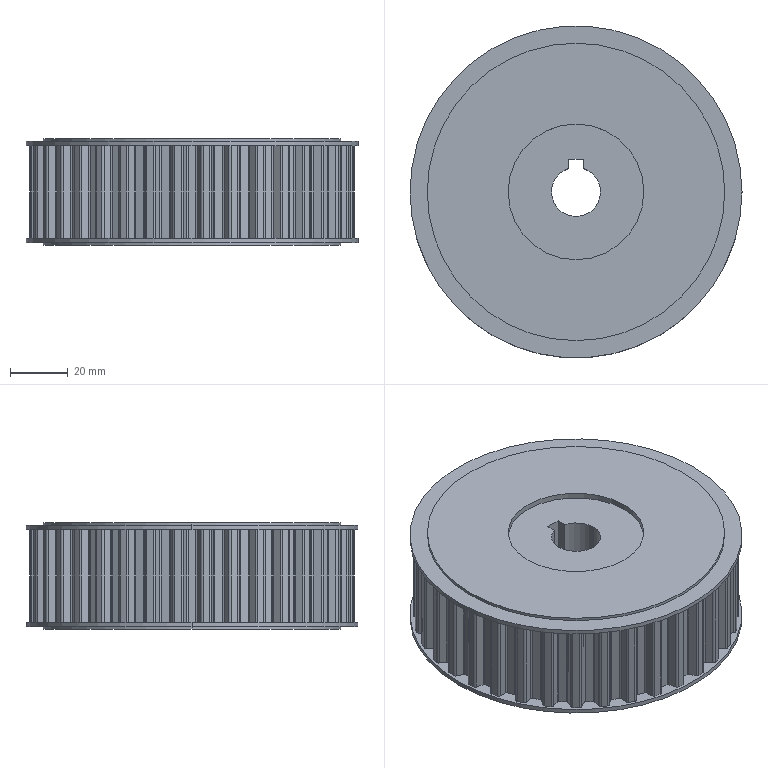Part | SolidWorks | features ICE 7, MirrorPattern 4, HoleWzd 2, CirPattern 1, Extrusion 1, RefAxis 1 | 1 solid | 349 faces | box 115 x 115 x 37 mm | volume 332155 mm3 | cylinder 227 | plane 120 | cone 2 | commonest cylinder face diameters 1.2 x86 1.6 x86 112.74 x36 47 x4 103 x4 115 x4